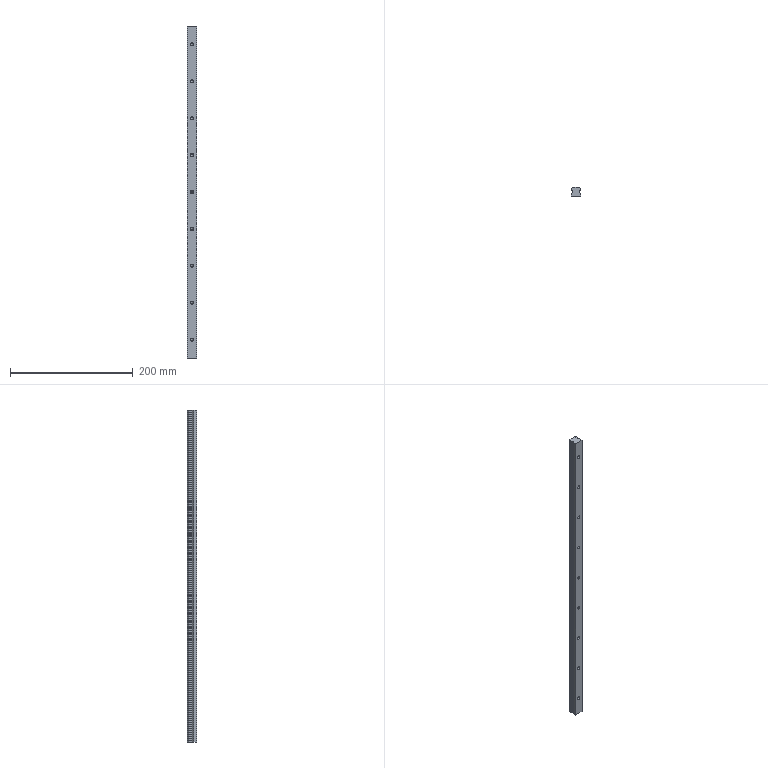Part | STEP file | 1 solid | 89 faces | box 15 x 15 x 540 mm | volume 107671 mm3 | cylinder 42 | plane 29 | cone 18 | commonest cylinder face diameters 4.25 x18 5 x18 1.459 x6